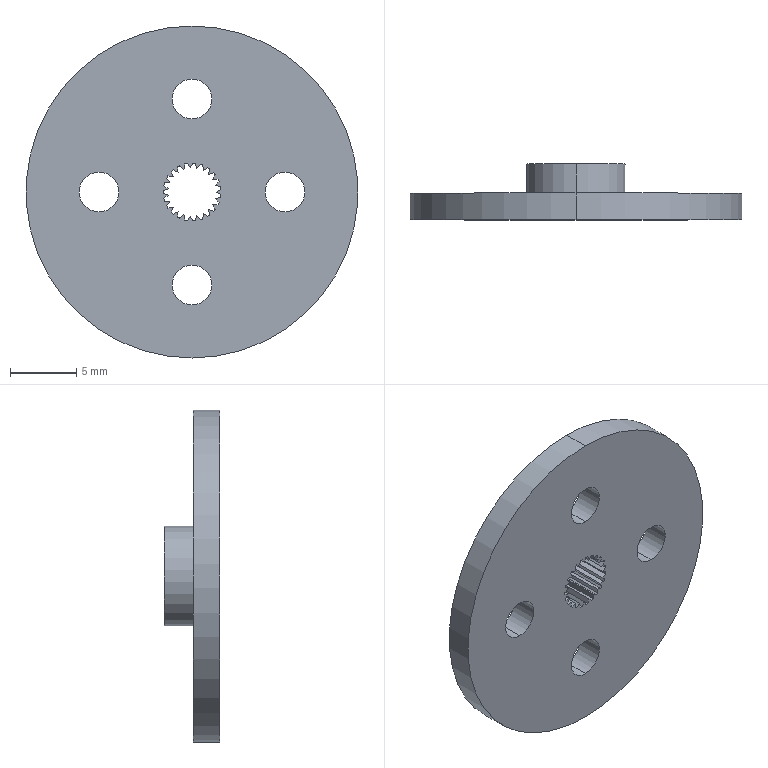Part | SolidWorks | features ICE 5, CirPattern 1, CombineBodies 1, Extrusion 1, MoveCopyBody 1, Stock 1 | 1 solid | 84 faces | box 25 x 4.2 x 25 mm | volume 966.612 mm3 | plane 49 | cylinder 35 | commonest cylinder face diameters 4.361 x23 3 x8 7.5 x2 25 x2